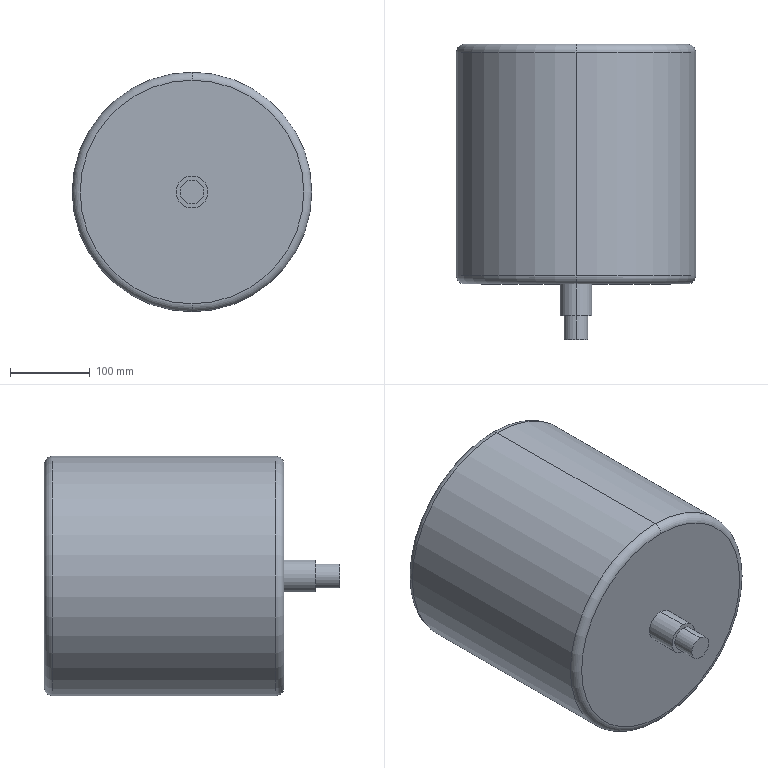Part | SolidWorks | features Fillet 1, Revolution 1 | 1 solid | 14 faces | box 300 x 370 x 300 mm | volume 21237373 mm3 | cylinder 6 | torus 4 | plane 4 | commonest cylinder face diameters 30 x2 40 x2 300 x2
STEP:
#1=CARTESIAN_POINT('',(0.,360.,-150.));
#2=VERTEX_POINT('',#1);
#3=CARTESIAN_POINT('',(0.,360.,150.));
#4=VERTEX_POINT('',#3);
#5=CARTESIAN_POINT('',(0.,360.,0.));
#6=DIRECTION('',(0.,-1.,0.));
#7=DIRECTION('',(0.,0.,1.));
#8=AXIS2_PLACEMENT_3D('',#5,#6,#7);
#9=CIRCLE('',#8,150.);
#10=EDGE_CURVE('',#2,#4,#9,.T.);
#11=ORIENTED_EDGE('',*,*,#10,.F.);
#12=CARTESIAN_POINT('',(0.,370.,-140.));
#13=VERTEX_POINT('',#12);
#14=CARTESIAN_POINT('',(0.,360.,-140.));
#15=DIRECTION('',(1.,0.,0.));
#16=DIRECTION('',(0.,0.,-1.));
#17=AXIS2_PLACEMENT_3D('',#14,#15,#16);
#18=CIRCLE('',#17,10.);
#19=EDGE_CURVE('',#2,#13,#18,.T.);
#20=ORIENTED_EDGE('',*,*,#19,.T.);
#21=CARTESIAN_POINT('',(0.,370.,140.));
#22=VERTEX_POINT('',#21);
#23=CARTESIAN_POINT('',(0.,370.,0.));
#24=DIRECTION('',(0.,1.,0.));
#25=DIRECTION('',(0.,0.,1.));
#26=AXIS2_PLACEMENT_3D('',#23,#24,#25);
#27=CIRCLE('',#26,140.);
#28=EDGE_CURVE('',#22,#13,#27,.T.);
#29=ORIENTED_EDGE('',*,*,#28,.F.);
#30=CARTESIAN_POINT('',(0.,360.,140.));
#31=DIRECTION('',(-1.,0.,0.));
#32=DIRECTION('',(0.,0.,1.));
#33=AXIS2_PLACEMENT_3D('',#30,#31,#32);
#34=CIRCLE('',#33,10.);
#35=EDGE_CURVE('',#4,#22,#34,.T.);
#36=ORIENTED_EDGE('',*,*,#35,.F.);
#37=EDGE_LOOP('',(#11,#20,#29,#36));
#38=FACE_OUTER_BOUND('',#37,.T.);
#39=CARTESIAN_POINT('',(0.,360.,0.));
#40=DIRECTION('',(0.,1.,0.));
#41=DIRECTION('',(0.,0.,1.));
#42=AXIS2_PLACEMENT_3D('',#39,#40,#41);
#43=TOROIDAL_SURFACE('',#42,140.,10.);
#44=ADVANCED_FACE('',(#38),#43,.T.);
#45=CARTESIAN_POINT('',(0.,80.,150.));
#46=VERTEX_POINT('',#45);
#47=CARTESIAN_POINT('',(0.,80.,-150.));
#48=VERTEX_POINT('',#47);
#49=CARTESIAN_POINT('',(0.,80.,0.));
#50=DIRECTION('',(0.,1.,0.));
#51=DIRECTION('',(0.,0.,-1.));
#52=AXIS2_PLACEMENT_3D('',#49,#50,#51);
#53=CIRCLE('',#52,150.);
#54=EDGE_CURVE('',#46,#48,#53,.T.);
#55=ORIENTED_EDGE('',*,*,#54,.F.);
#56=CARTESIAN_POINT('',(0.,70.,140.));
#57=VERTEX_POINT('',#56);
#58=CARTESIAN_POINT('',(0.,80.,140.));
#59=DIRECTION('',(1.,0.,0.));
#60=DIRECTION('',(0.,0.,-1.));
#61=AXIS2_PLACEMENT_3D('',#58,#59,#60);
#62=CIRCLE('',#61,10.);
#63=EDGE_CURVE('',#46,#57,#62,.T.);
#64=ORIENTED_EDGE('',*,*,#63,.T.);
#65=CARTESIAN_POINT('',(0.,70.,-140.));
#66=VERTEX_POINT('',#65);
#67=CARTESIAN_POINT('',(0.,70.,0.));
#68=DIRECTION('',(0.,-1.,0.));
#69=DIRECTION('',(0.,0.,-1.));
#70=AXIS2_PLACEMENT_3D('',#67,#68,#69);
#71=CIRCLE('',#70,140.);
#72=EDGE_CURVE('',#66,#57,#71,.T.);
#73=ORIENTED_EDGE('',*,*,#72,.F.);
#74=CARTESIAN_POINT('',(0.,80.,-140.));
#75=DIRECTION('',(-1.,0.,0.));
#76=DIRECTION('',(0.,0.,1.));
#77=AXIS2_PLACEMENT_3D('',#74,#75,#76);
#78=CIRCLE('',#77,10.);
#79=EDGE_CURVE('',#48,#66,#78,.T.);
#80=ORIENTED_EDGE('',*,*,#79,.F.);
#81=EDGE_LOOP('',(#55,#64,#73,#80));
#82=FACE_OUTER_BOUND('',#81,.T.);
#83=CARTESIAN_POINT('',(0.,80.,0.));
#84=DIRECTION('',(0.,-1.,0.));
#85=DIRECTION('',(0.,0.,-1.));
#86=AXIS2_PLACEMENT_3D('',#83,#84,#85);
#87=TOROIDAL_SURFACE('',#86,140.,10.);
#88=ADVANCED_FACE('',(#82),#87,.T.);
#89=CARTESIAN_POINT('',(0.,30.,-15.));
#90=VERTEX_POINT('',#89);
#91=CARTESIAN_POINT('',(0.,30.,15.));
#92=VERTEX_POINT('',#91);
#93=CARTESIAN_POINT('',(0.,30.,0.));
#94=DIRECTION('',(0.,-1.,0.));
#95=DIRECTION('',(0.,0.,-1.));
#96=AXIS2_PLACEMENT_3D('',#93,#94,#95);
#97=CIRCLE('',#96,15.);
#98=EDGE_CURVE('',#90,#92,#97,.T.);
#99=ORIENTED_EDGE('',*,*,#98,.T.);
#100=CARTESIAN_POINT('',(0.,0.,15.));
#101=VERTEX_POINT('',#100);
#102=CARTESIAN_POINT('',(0.,0.,15.));
#103=DIRECTION('',(0.,-1.,0.));
#104=VECTOR('',#103,1000.);
#105=LINE('',#102,#104);
#106=EDGE_CURVE('',#92,#101,#105,.T.);
#107=ORIENTED_EDGE('',*,*,#106,.T.);
#108=CARTESIAN_POINT('',(0.,0.,-15.));
#109=VERTEX_POINT('',#108);
#110=CARTESIAN_POINT('',(0.,0.,0.));
#111=DIRECTION('',(0.,-1.,0.));
#112=DIRECTION('',(0.,0.,-1.));
#113=AXIS2_PLACEMENT_3D('',#110,#111,#112);
#114=CIRCLE('',#113,15.);
#115=EDGE_CURVE('',#109,#101,#114,.T.);
#116=ORIENTED_EDGE('',*,*,#115,.F.);
#117=CARTESIAN_POINT('',(0.,0.,-15.));
#118=DIRECTION('',(0.,-1.,0.));
#119=VECTOR('',#118,1000.);
#120=LINE('',#117,#119);
#121=EDGE_CURVE('',#90,#109,#120,.T.);
#122=ORIENTED_EDGE('',*,*,#121,.F.);
#123=EDGE_LOOP('',(#99,#107,#116,#122));
#124=FACE_OUTER_BOUND('',#123,.T.);
#125=CARTESIAN_POINT('',(0.,0.,0.));
#126=DIRECTION('',(0.,-1.,0.));
#127=DIRECTION('',(0.,0.,-1.));
#128=AXIS2_PLACEMENT_3D('',#125,#126,#127);
#129=CYLINDRICAL_SURFACE('',#128,15.);
#130=ADVANCED_FACE('',(#124),#129,.T.);
#131=CARTESIAN_POINT('',(0.,70.,-20.));
#132=VERTEX_POINT('',#131);
#133=CARTESIAN_POINT('',(0.,70.,20.));
#134=VERTEX_POINT('',#133);
#135=CARTESIAN_POINT('',(0.,70.,0.));
#136=DIRECTION('',(0.,-1.,0.));
#137=DIRECTION('',(0.,0.,-1.));
#138=AXIS2_PLACEMENT_3D('',#135,#136,#137);
#139=CIRCLE('',#138,20.);
#140=EDGE_CURVE('',#132,#134,#139,.T.);
#141=ORIENTED_EDGE('',*,*,#140,.T.);
#142=CARTESIAN_POINT('',(0.,30.,20.));
#143=VERTEX_POINT('',#142);
#144=CARTESIAN_POINT('',(0.,0.,20.));
#145=DIRECTION('',(0.,-1.,0.));
#146=VECTOR('',#145,1000.);
#147=LINE('',#144,#146);
#148=EDGE_CURVE('',#134,#143,#147,.T.);
#149=ORIENTED_EDGE('',*,*,#148,.T.);
#150=CARTESIAN_POINT('',(0.,30.,-20.));
#151=VERTEX_POINT('',#150);
#152=CARTESIAN_POINT('',(0.,30.,0.));
#153=DIRECTION('',(0.,-1.,0.));
#154=DIRECTION('',(0.,0.,-1.));
#155=AXIS2_PLACEMENT_3D('',#152,#153,#154);
#156=CIRCLE('',#155,20.);
#157=EDGE_CURVE('',#151,#143,#156,.T.);
#158=ORIENTED_EDGE('',*,*,#157,.F.);
#159=CARTESIAN_POINT('',(0.,0.,-20.));
#160=DIRECTION('',(0.,-1.,0.));
#161=VECTOR('',#160,1000.);
#162=LINE('',#159,#161);
#163=EDGE_CURVE('',#132,#151,#162,.T.);
#164=ORIENTED_EDGE('',*,*,#163,.F.);
#165=EDGE_LOOP('',(#141,#149,#158,#164));
#166=FACE_OUTER_BOUND('',#165,.T.);
#167=CARTESIAN_POINT('',(0.,0.,0.));
#168=DIRECTION('',(0.,-1.,0.));
#169=DIRECTION('',(0.,0.,-1.));
#170=AXIS2_PLACEMENT_3D('',#167,#168,#169);
#171=CYLINDRICAL_SURFACE('',#170,20.);
#172=ADVANCED_FACE('',(#166),#171,.T.);
#173=ORIENTED_EDGE('',*,*,#10,.T.);
#174=CARTESIAN_POINT('',(0.,0.,150.));
#175=DIRECTION('',(0.,-1.,0.));
#176=VECTOR('',#175,1000.);
#177=LINE('',#174,#176);
#178=EDGE_CURVE('',#4,#46,#177,.T.);
#179=ORIENTED_EDGE('',*,*,#178,.T.);
#180=ORIENTED_EDGE('',*,*,#54,.T.);
#181=CARTESIAN_POINT('',(0.,0.,-150.));
#182=DIRECTION('',(0.,-1.,0.));
#183=VECTOR('',#182,1000.);
#184=LINE('',#181,#183);
#185=EDGE_CURVE('',#2,#48,#184,.T.);
#186=ORIENTED_EDGE('',*,*,#185,.F.);
#187=EDGE_LOOP('',(#173,#179,#180,#186));
#188=FACE_OUTER_BOUND('',#187,.T.);
#189=CARTESIAN_POINT('',(0.,0.,0.));
#190=DIRECTION('',(0.,-1.,0.));
#191=DIRECTION('',(0.,0.,-1.));
#192=AXIS2_PLACEMENT_3D('',#189,#190,#191);
#193=CYLINDRICAL_SURFACE('',#192,150.);
#194=ADVANCED_FACE('',(#188),#193,.T.);
#195=ORIENTED_EDGE('',*,*,#115,.T.);
#196=CARTESIAN_POINT('',(0.,0.,0.));
#197=DIRECTION('',(0.,-1.,0.));
#198=DIRECTION('',(0.,0.,-1.));
#199=AXIS2_PLACEMENT_3D('',#196,#197,#198);
#200=CIRCLE('',#199,15.);
#201=EDGE_CURVE('',#101,#109,#200,.T.);
#202=ORIENTED_EDGE('',*,*,#201,.T.);
#203=EDGE_LOOP('',(#195,#202));
#204=FACE_OUTER_BOUND('',#203,.T.);
#205=CARTESIAN_POINT('',(15.,0.,0.));
#206=DIRECTION('',(0.,-1.,0.));
#207=DIRECTION('',(0.,0.,-1.));
#208=AXIS2_PLACEMENT_3D('',#205,#206,#207);
#209=PLANE('',#208);
#210=ADVANCED_FACE('',(#204),#209,.T.);
#211=ORIENTED_EDGE('',*,*,#28,.T.);
#212=CARTESIAN_POINT('',(0.,370.,0.));
#213=DIRECTION('',(0.,1.,0.));
#214=DIRECTION('',(0.,0.,1.));
#215=AXIS2_PLACEMENT_3D('',#212,#213,#214);
#216=CIRCLE('',#215,140.);
#217=EDGE_CURVE('',#13,#22,#216,.T.);
#218=ORIENTED_EDGE('',*,*,#217,.T.);
#219=EDGE_LOOP('',(#211,#218));
#220=FACE_OUTER_BOUND('',#219,.T.);
#221=CARTESIAN_POINT('',(0.,370.,0.));
#222=DIRECTION('',(0.,1.,0.));
#223=DIRECTION('',(0.,0.,1.));
#224=AXIS2_PLACEMENT_3D('',#221,#222,#223);
#225=PLANE('',#224);
#226=ADVANCED_FACE('',(#220),#225,.T.);
#227=ORIENTED_EDGE('',*,*,#178,.F.);
#228=CARTESIAN_POINT('',(0.,360.,0.));
#229=DIRECTION('',(0.,-1.,0.));
#230=DIRECTION('',(0.,0.,1.));
#231=AXIS2_PLACEMENT_3D('',#228,#229,#230);
#232=CIRCLE('',#231,150.);
#233=EDGE_CURVE('',#4,#2,#232,.T.);
#234=ORIENTED_EDGE('',*,*,#233,.T.);
#235=ORIENTED_EDGE('',*,*,#185,.T.);
#236=CARTESIAN_POINT('',(0.,80.,0.));
#237=DIRECTION('',(0.,1.,0.));
#238=DIRECTION('',(0.,0.,-1.));
#239=AXIS2_PLACEMENT_3D('',#236,#237,#238);
#240=CIRCLE('',#239,150.);
#241=EDGE_CURVE('',#48,#46,#240,.T.);
#242=ORIENTED_EDGE('',*,*,#241,.T.);
#243=EDGE_LOOP('',(#227,#234,#235,#242));
#244=FACE_OUTER_BOUND('',#243,.T.);
#245=CARTESIAN_POINT('',(0.,0.,0.));
#246=DIRECTION('',(0.,-1.,0.));
#247=DIRECTION('',(0.,0.,-1.));
#248=AXIS2_PLACEMENT_3D('',#245,#246,#247);
#249=CYLINDRICAL_SURFACE('',#248,150.);
#250=ADVANCED_FACE('',(#244),#249,.T.);
#251=ORIENTED_EDGE('',*,*,#72,.T.);
#252=CARTESIAN_POINT('',(0.,70.,0.));
#253=DIRECTION('',(0.,-1.,0.));
#254=DIRECTION('',(0.,0.,-1.));
#255=AXIS2_PLACEMENT_3D('',#252,#253,#254);
#256=CIRCLE('',#255,140.);
#257=EDGE_CURVE('',#57,#66,#256,.T.);
#258=ORIENTED_EDGE('',*,*,#257,.T.);
#259=EDGE_LOOP('',(#251,#258));
#260=FACE_OUTER_BOUND('',#259,.T.);
#261=ORIENTED_EDGE('',*,*,#140,.F.);
#262=CARTESIAN_POINT('',(0.,70.,0.));
#263=DIRECTION('',(0.,-1.,0.));
#264=DIRECTION('',(0.,0.,-1.));
#265=AXIS2_PLACEMENT_3D('',#262,#263,#264);
#266=CIRCLE('',#265,20.);
#267=EDGE_CURVE('',#134,#132,#266,.T.);
#268=ORIENTED_EDGE('',*,*,#267,.F.);
#269=EDGE_LOOP('',(#261,#268));
#270=FACE_BOUND('',#269,.T.);
#271=CARTESIAN_POINT('',(150.,70.,0.));
#272=DIRECTION('',(0.,-1.,0.));
#273=DIRECTION('',(0.,0.,-1.));
#274=AXIS2_PLACEMENT_3D('',#271,#272,#273);
#275=PLANE('',#274);
#276=ADVANCED_FACE('',(#260,#270),#275,.T.);
#277=ORIENTED_EDGE('',*,*,#148,.F.);
#278=ORIENTED_EDGE('',*,*,#267,.T.);
#279=ORIENTED_EDGE('',*,*,#163,.T.);
#280=CARTESIAN_POINT('',(0.,30.,0.));
#281=DIRECTION('',(0.,-1.,0.));
#282=DIRECTION('',(0.,0.,-1.));
#283=AXIS2_PLACEMENT_3D('',#280,#281,#282);
#284=CIRCLE('',#283,20.);
#285=EDGE_CURVE('',#143,#151,#284,.T.);
#286=ORIENTED_EDGE('',*,*,#285,.F.);
#287=EDGE_LOOP('',(#277,#278,#279,#286));
#288=FACE_OUTER_BOUND('',#287,.T.);
#289=CARTESIAN_POINT('',(0.,0.,0.));
#290=DIRECTION('',(0.,-1.,0.));
#291=DIRECTION('',(0.,0.,-1.));
#292=AXIS2_PLACEMENT_3D('',#289,#290,#291);
#293=CYLINDRICAL_SURFACE('',#292,20.);
#294=ADVANCED_FACE('',(#288),#293,.T.);
#295=ORIENTED_EDGE('',*,*,#157,.T.);
#296=ORIENTED_EDGE('',*,*,#285,.T.);
#297=EDGE_LOOP('',(#295,#296));
#298=FACE_OUTER_BOUND('',#297,.T.);
#299=ORIENTED_EDGE('',*,*,#98,.F.);
#300=CARTESIAN_POINT('',(0.,30.,0.));
#301=DIRECTION('',(0.,-1.,0.));
#302=DIRECTION('',(0.,0.,-1.));
#303=AXIS2_PLACEMENT_3D('',#300,#301,#302);
#304=CIRCLE('',#303,15.);
#305=EDGE_CURVE('',#92,#90,#304,.T.);
#306=ORIENTED_EDGE('',*,*,#305,.F.);
#307=EDGE_LOOP('',(#299,#306));
#308=FACE_BOUND('',#307,.T.);
#309=CARTESIAN_POINT('',(20.,30.,0.));
#310=DIRECTION('',(0.,-1.,0.));
#311=DIRECTION('',(0.,0.,-1.));
#312=AXIS2_PLACEMENT_3D('',#309,#310,#311);
#313=PLANE('',#312);
#314=ADVANCED_FACE('',(#298,#308),#313,.T.);
#315=ORIENTED_EDGE('',*,*,#106,.F.);
#316=ORIENTED_EDGE('',*,*,#305,.T.);
#317=ORIENTED_EDGE('',*,*,#121,.T.);
#318=ORIENTED_EDGE('',*,*,#201,.F.);
#319=EDGE_LOOP('',(#315,#316,#317,#318));
#320=FACE_OUTER_BOUND('',#319,.T.);
#321=CARTESIAN_POINT('',(0.,0.,0.));
#322=DIRECTION('',(0.,-1.,0.));
#323=DIRECTION('',(0.,0.,-1.));
#324=AXIS2_PLACEMENT_3D('',#321,#322,#323);
#325=CYLINDRICAL_SURFACE('',#324,15.);
#326=ADVANCED_FACE('',(#320),#325,.T.);
#327=ORIENTED_EDGE('',*,*,#63,.F.);
#328=ORIENTED_EDGE('',*,*,#241,.F.);
#329=ORIENTED_EDGE('',*,*,#79,.T.);
#330=ORIENTED_EDGE('',*,*,#257,.F.);
#331=EDGE_LOOP('',(#327,#328,#329,#330));
#332=FACE_OUTER_BOUND('',#331,.T.);
#333=CARTESIAN_POINT('',(0.,80.,0.));
#334=DIRECTION('',(0.,-1.,0.));
#335=DIRECTION('',(0.,0.,-1.));
#336=AXIS2_PLACEMENT_3D('',#333,#334,#335);
#337=TOROIDAL_SURFACE('',#336,140.,10.);
#338=ADVANCED_FACE('',(#332),#337,.T.);
#339=ORIENTED_EDGE('',*,*,#19,.F.);
#340=ORIENTED_EDGE('',*,*,#233,.F.);
#341=ORIENTED_EDGE('',*,*,#35,.T.);
#342=ORIENTED_EDGE('',*,*,#217,.F.);
#343=EDGE_LOOP('',(#339,#340,#341,#342));
#344=FACE_OUTER_BOUND('',#343,.T.);
#345=CARTESIAN_POINT('',(0.,360.,0.));
#346=DIRECTION('',(0.,1.,0.));
#347=DIRECTION('',(0.,0.,1.));
#348=AXIS2_PLACEMENT_3D('',#345,#346,#347);
#349=TOROIDAL_SURFACE('',#348,140.,10.);
#350=ADVANCED_FACE('',(#344),#349,.T.);
#351=CLOSED_SHELL('',(#44,#88,#130,#172,#194,#210,#226,#250,#276,#294,#314,#326,#338,#350));
#352=MANIFOLD_SOLID_BREP('',#351);
#353=CARTESIAN_POINT('',(0.,0.,0.));
#354=DIRECTION('',(0.,0.,1.));
#355=DIRECTION('',(1.,0.,0.));
#356=AXIS2_PLACEMENT_3D('',#353,#354,#355);
#357=(LENGTH_UNIT()NAMED_UNIT(*)SI_UNIT(.MILLI.,.METRE.));
#358=UNCERTAINTY_MEASURE_WITH_UNIT(LENGTH_MEASURE(0.00001),#357,'','');
#359=(NAMED_UNIT(*)PLANE_ANGLE_UNIT()SI_UNIT($,.RADIAN.));
#360=(NAMED_UNIT(*)SI_UNIT($,.STERADIAN.)SOLID_ANGLE_UNIT());
#361=(GEOMETRIC_REPRESENTATION_CONTEXT(3)GLOBAL_UNCERTAINTY_ASSIGNED_CONTEXT((#358))GLOBAL_UNIT_ASSIGNED_CONTEXT((#357,#359,#360))REPRESENTATION_CONTEXT('',''));
#362=ADVANCED_BREP_SHAPE_REPRESENTATION('',(#352,#356),#361);